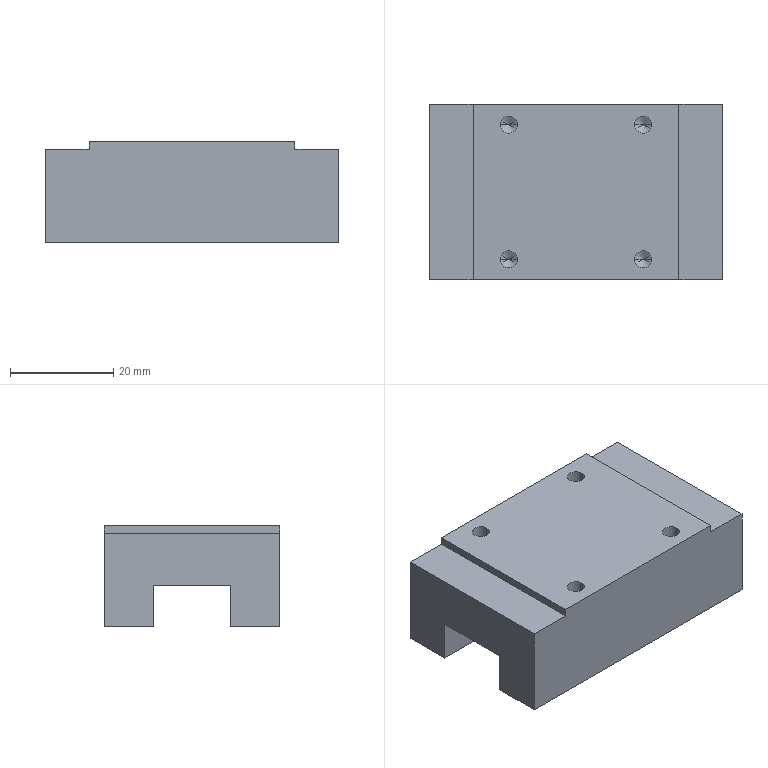Part | STEP file | Bag feed EGH15CA slider | 1 solid | 30 faces | box 56.8 x 34 x 19.5 mm | volume 29571 mm3 | plane 14 | cylinder 8 | cone 8 | commonest cylinder face diameters 3.3 x8